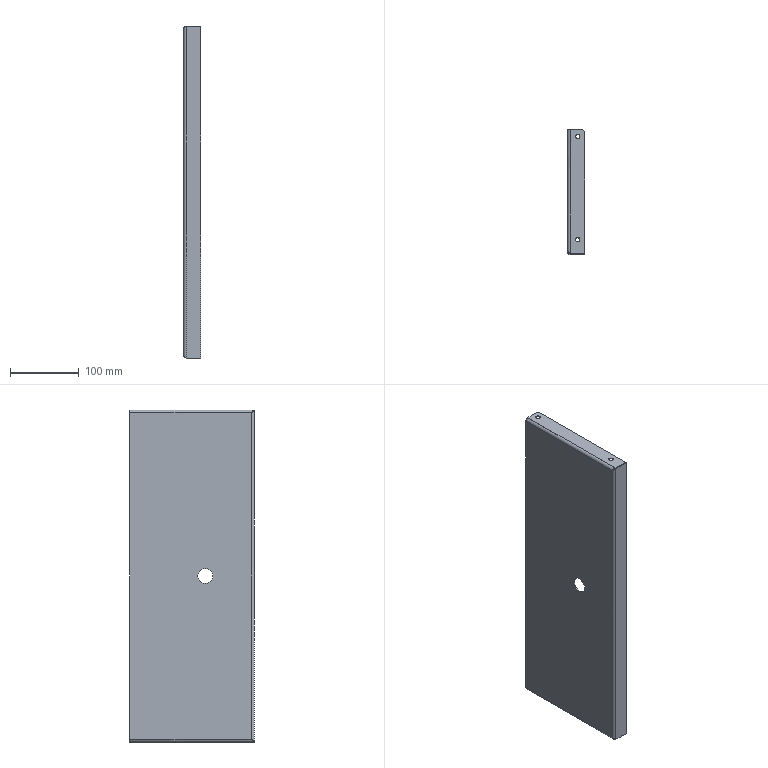Part | STEP file | 21-Motor cover plate | 1 solid | 42 faces | box 25 x 181 x 482 mm | volume 105638 mm3 | plane 20 | cylinder 18 | spline 4 | commonest cylinder face diameters 6.6 x8 6 x3 8 x3 10 x2 22 x2